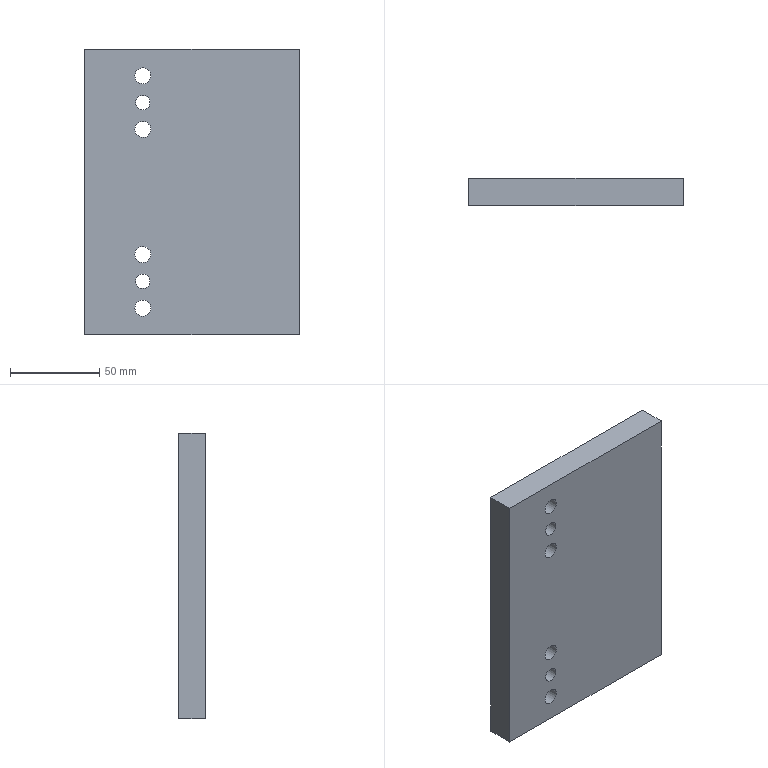Part | STEP file | Copy (1) of SN10_008_007-02_PLACA | 1 solid | 12 faces | box 120 x 15 x 160 mm | volume 282675 mm3 | cylinder 6 | plane 6 | commonest cylinder face diameters 9 x4 8 x2
STEP:
#1=CARTESIAN_POINT('',(0.,0.,0.));
#2=DIRECTION('',(0.,0.,1.));
#3=DIRECTION('',(1.,0.,0.));
#4=AXIS2_PLACEMENT_3D('',#1,#2,#3);
#5=CARTESIAN_POINT('',(279.639,240.,404.352));
#6=VERTEX_POINT('',#5);
#7=CARTESIAN_POINT('',(276.129,240.,406.27));
#8=DIRECTION('',(0.,-1.,0.));
#9=DIRECTION('',(1.,0.,0.));
#10=AXIS2_PLACEMENT_3D('',#7,#8,#9);
#11=CIRCLE('',#10,4.);
#12=CARTESIAN_POINT('',(276.129,240.1,406.27));
#13=DIRECTION('',(0.,1.,0.));
#14=DIRECTION('',(0.8776,0.,-0.4794));
#15=AXIS2_PLACEMENT_3D('',#12,#13,#14);
#16=CYLINDRICAL_SURFACE('',#15,4.);
#17=CARTESIAN_POINT('',(12.066,-0.1));
#18=DIRECTION('',(-1.,0.));
#19=VECTOR('',#18,1.);
#20=LINE('',#17,#19);
#21=(GEOMETRIC_REPRESENTATION_CONTEXT(2)PARAMETRIC_REPRESENTATION_CONTEXT()REPRESENTATION_CONTEXT('',''));
#22=DEFINITIONAL_REPRESENTATION('',(#20),#21);
#23=PCURVE('',#16,#22);
#24=CARTESIAN_POINT('',(363.629,240.,446.));
#25=DIRECTION('',(0.,-1.,0.));
#26=DIRECTION('',(0.,0.,-1.));
#27=AXIS2_PLACEMENT_3D('',#24,#25,#26);
#28=PLANE('',#27);
#29=CARTESIAN_POINT('',(39.73,-87.5));
#30=DIRECTION('',(0.,1.));
#31=AXIS2_PLACEMENT_2D('',#29,#30);
#32=CIRCLE('',#31,4.);
#33=(GEOMETRIC_REPRESENTATION_CONTEXT(2)PARAMETRIC_REPRESENTATION_CONTEXT()REPRESENTATION_CONTEXT('',''));
#34=DEFINITIONAL_REPRESENTATION('',(#32),#33);
#35=PCURVE('',#28,#34);
#36=SURFACE_CURVE('',#11,(#23,#35),.PCURVE_S1.);
#37=EDGE_CURVE('',#6,#6,#36,.T.);
#38=ORIENTED_EDGE('',*,*,#37,.F.);
#39=CARTESIAN_POINT('',(279.639,255.,404.352));
#40=VERTEX_POINT('',#39);
#41=CARTESIAN_POINT('',(279.639,240.,404.352));
#42=CARTESIAN_POINT('',(279.639,255.,404.352));
#43=B_SPLINE_CURVE_WITH_KNOTS('',1,(#41,#42),.UNSPECIFIED.,.F.,.F.,(2,2),(-0.1,14.9),.PIECEWISE_BEZIER_KNOTS.);
#44=CARTESIAN_POINT('',(6.283,0.));
#45=DIRECTION('',(0.,1.));
#46=VECTOR('',#45,1.);
#47=LINE('',#44,#46);
#48=(GEOMETRIC_REPRESENTATION_CONTEXT(2)PARAMETRIC_REPRESENTATION_CONTEXT()REPRESENTATION_CONTEXT('',''));
#49=DEFINITIONAL_REPRESENTATION('',(#47),#48);
#50=PCURVE('',#16,#49);
#51=CARTESIAN_POINT('',(0.,0.));
#52=DIRECTION('',(0.,1.));
#53=VECTOR('',#52,1.);
#54=LINE('',#51,#53);
#55=(GEOMETRIC_REPRESENTATION_CONTEXT(2)PARAMETRIC_REPRESENTATION_CONTEXT()REPRESENTATION_CONTEXT('',''));
#56=DEFINITIONAL_REPRESENTATION('',(#54),#55);
#57=PCURVE('',#16,#56);
#58=SEAM_CURVE('',#43,(#50,#57),.PCURVE_S1.);
#59=EDGE_CURVE('',#6,#40,#58,.T.);
#60=ORIENTED_EDGE('',*,*,#59,.T.);
#61=CARTESIAN_POINT('',(276.129,255.,406.27));
#62=DIRECTION('',(0.,1.,0.));
#63=DIRECTION('',(1.,0.,0.));
#64=AXIS2_PLACEMENT_3D('',#61,#62,#63);
#65=CIRCLE('',#64,4.);
#66=CARTESIAN_POINT('',(-0.5,14.9));
#67=DIRECTION('',(1.,0.));
#68=VECTOR('',#67,1.);
#69=LINE('',#66,#68);
#70=(GEOMETRIC_REPRESENTATION_CONTEXT(2)PARAMETRIC_REPRESENTATION_CONTEXT()REPRESENTATION_CONTEXT('',''));
#71=DEFINITIONAL_REPRESENTATION('',(#69),#70);
#72=PCURVE('',#16,#71);
#73=CARTESIAN_POINT('',(243.629,255.,446.));
#74=DIRECTION('',(0.,1.,0.));
#75=DIRECTION('',(0.,0.,1.));
#76=AXIS2_PLACEMENT_3D('',#73,#74,#75);
#77=PLANE('',#76);
#78=CARTESIAN_POINT('',(-39.73,32.5));
#79=DIRECTION('',(0.,1.));
#80=AXIS2_PLACEMENT_2D('',#78,#79);
#81=CIRCLE('',#80,4.);
#82=(GEOMETRIC_REPRESENTATION_CONTEXT(2)PARAMETRIC_REPRESENTATION_CONTEXT()REPRESENTATION_CONTEXT('',''));
#83=DEFINITIONAL_REPRESENTATION('',(#81),#82);
#84=PCURVE('',#77,#83);
#85=SURFACE_CURVE('',#65,(#72,#84),.PCURVE_S1.);
#86=EDGE_CURVE('',#40,#40,#85,.T.);
#87=ORIENTED_EDGE('',*,*,#86,.F.);
#88=ORIENTED_EDGE('',*,*,#59,.F.);
#89=EDGE_LOOP('',(#38,#60,#87,#88));
#90=FACE_BOUND('',#89,.F.);
#91=ADVANCED_FACE('',(#90),#16,.F.);
#92=CARTESIAN_POINT('',(243.629,240.,436.27));
#93=VERTEX_POINT('',#92);
#94=CARTESIAN_POINT('',(243.629,240.,276.27));
#95=VERTEX_POINT('',#94);
#96=CARTESIAN_POINT('',(243.629,240.,436.27));
#97=DIRECTION('',(0.,0.,-1.));
#98=VECTOR('',#97,1.);
#99=LINE('',#96,#98);
#100=CARTESIAN_POINT('',(9.73,-120.));
#101=DIRECTION('',(1.,0.));
#102=VECTOR('',#101,1.);
#103=LINE('',#100,#102);
#104=(GEOMETRIC_REPRESENTATION_CONTEXT(2)PARAMETRIC_REPRESENTATION_CONTEXT()REPRESENTATION_CONTEXT('',''));
#105=DEFINITIONAL_REPRESENTATION('',(#103),#104);
#106=PCURVE('',#28,#105);
#107=CARTESIAN_POINT('',(243.629,255.,446.));
#108=DIRECTION('',(1.,0.,0.));
#109=DIRECTION('',(0.,0.,-1.));
#110=AXIS2_PLACEMENT_3D('',#107,#108,#109);
#111=PLANE('',#110);
#112=CARTESIAN_POINT('',(9.73,-15.));
#113=DIRECTION('',(1.,0.));
#114=VECTOR('',#113,1.);
#115=LINE('',#112,#114);
#116=(GEOMETRIC_REPRESENTATION_CONTEXT(2)PARAMETRIC_REPRESENTATION_CONTEXT()REPRESENTATION_CONTEXT('',''));
#117=DEFINITIONAL_REPRESENTATION('',(#115),#116);
#118=PCURVE('',#111,#117);
#119=SURFACE_CURVE('',#99,(#106,#118),.PCURVE_S1.);
#120=EDGE_CURVE('',#93,#95,#119,.T.);
#121=ORIENTED_EDGE('',*,*,#120,.T.);
#122=CARTESIAN_POINT('',(363.629,240.,276.27));
#123=VERTEX_POINT('',#122);
#124=CARTESIAN_POINT('',(363.629,240.,276.27));
#125=DIRECTION('',(-1.,0.,0.));
#126=VECTOR('',#125,1.);
#127=LINE('',#124,#126);
#128=CARTESIAN_POINT('',(169.73,0.));
#129=DIRECTION('',(0.,-1.));
#130=VECTOR('',#129,1.);
#131=LINE('',#128,#130);
#132=(GEOMETRIC_REPRESENTATION_CONTEXT(2)PARAMETRIC_REPRESENTATION_CONTEXT()REPRESENTATION_CONTEXT('',''));
#133=DEFINITIONAL_REPRESENTATION('',(#131),#132);
#134=PCURVE('',#28,#133);
#135=CARTESIAN_POINT('',(243.629,270.,276.27));
#136=DIRECTION('',(0.,0.,-1.));
#137=DIRECTION('',(-1.,0.,0.));
#138=AXIS2_PLACEMENT_3D('',#135,#136,#137);
#139=PLANE('',#138);
#140=CARTESIAN_POINT('',(-120.,-30.));
#141=DIRECTION('',(1.,0.));
#142=VECTOR('',#141,1.);
#143=LINE('',#140,#142);
#144=(GEOMETRIC_REPRESENTATION_CONTEXT(2)PARAMETRIC_REPRESENTATION_CONTEXT()REPRESENTATION_CONTEXT('',''));
#145=DEFINITIONAL_REPRESENTATION('',(#143),#144);
#146=PCURVE('',#139,#145);
#147=SURFACE_CURVE('',#127,(#134,#146),.PCURVE_S1.);
#148=EDGE_CURVE('',#123,#95,#147,.T.);
#149=ORIENTED_EDGE('',*,*,#148,.F.);
#150=CARTESIAN_POINT('',(363.629,240.,436.27));
#151=VERTEX_POINT('',#150);
#152=CARTESIAN_POINT('',(363.629,240.,436.27));
#153=DIRECTION('',(0.,0.,-1.));
#154=VECTOR('',#153,1.);
#155=LINE('',#152,#154);
#156=CARTESIAN_POINT('',(9.73,0.));
#157=DIRECTION('',(1.,0.));
#158=VECTOR('',#157,1.);
#159=LINE('',#156,#158);
#160=(GEOMETRIC_REPRESENTATION_CONTEXT(2)PARAMETRIC_REPRESENTATION_CONTEXT()REPRESENTATION_CONTEXT('',''));
#161=DEFINITIONAL_REPRESENTATION('',(#159),#160);
#162=PCURVE('',#28,#161);
#163=CARTESIAN_POINT('',(363.629,240.,446.));
#164=DIRECTION('',(-1.,0.,0.));
#165=DIRECTION('',(0.,0.,1.));
#166=AXIS2_PLACEMENT_3D('',#163,#164,#165);
#167=PLANE('',#166);
#168=CARTESIAN_POINT('',(-9.73,0.));
#169=DIRECTION('',(-1.,0.));
#170=VECTOR('',#169,1.);
#171=LINE('',#168,#170);
#172=(GEOMETRIC_REPRESENTATION_CONTEXT(2)PARAMETRIC_REPRESENTATION_CONTEXT()REPRESENTATION_CONTEXT('',''));
#173=DEFINITIONAL_REPRESENTATION('',(#171),#172);
#174=PCURVE('',#167,#173);
#175=SURFACE_CURVE('',#155,(#162,#174),.PCURVE_S1.);
#176=EDGE_CURVE('',#151,#123,#175,.T.);
#177=ORIENTED_EDGE('',*,*,#176,.F.);
#178=CARTESIAN_POINT('',(363.629,240.,436.27));
#179=DIRECTION('',(-1.,0.,0.));
#180=VECTOR('',#179,1.);
#181=LINE('',#178,#180);
#182=CARTESIAN_POINT('',(9.73,0.));
#183=DIRECTION('',(0.,-1.));
#184=VECTOR('',#183,1.);
#185=LINE('',#182,#184);
#186=(GEOMETRIC_REPRESENTATION_CONTEXT(2)PARAMETRIC_REPRESENTATION_CONTEXT()REPRESENTATION_CONTEXT('',''));
#187=DEFINITIONAL_REPRESENTATION('',(#185),#186);
#188=PCURVE('',#28,#187);
#189=CARTESIAN_POINT('',(243.629,255.,436.27));
#190=DIRECTION('',(0.,0.,1.));
#191=DIRECTION('',(1.,0.,0.));
#192=AXIS2_PLACEMENT_3D('',#189,#190,#191);
#193=PLANE('',#192);
#194=CARTESIAN_POINT('',(120.,-15.));
#195=DIRECTION('',(-1.,0.));
#196=VECTOR('',#195,1.);
#197=LINE('',#194,#196);
#198=(GEOMETRIC_REPRESENTATION_CONTEXT(2)PARAMETRIC_REPRESENTATION_CONTEXT()REPRESENTATION_CONTEXT('',''));
#199=DEFINITIONAL_REPRESENTATION('',(#197),#198);
#200=PCURVE('',#193,#199);
#201=SURFACE_CURVE('',#181,(#188,#200),.PCURVE_S1.);
#202=EDGE_CURVE('',#151,#93,#201,.T.);
#203=ORIENTED_EDGE('',*,*,#202,.T.);
#204=EDGE_LOOP('',(#121,#149,#177,#203));
#205=FACE_BOUND('',#204,.T.);
#206=ORIENTED_EDGE('',*,*,#37,.F.);
#207=EDGE_LOOP('',(#206));
#208=FACE_BOUND('',#207,.T.);
#209=CARTESIAN_POINT('',(279.639,240.,304.352));
#210=VERTEX_POINT('',#209);
#211=CARTESIAN_POINT('',(276.129,240.,306.27));
#212=DIRECTION('',(0.,-1.,0.));
#213=DIRECTION('',(1.,0.,0.));
#214=AXIS2_PLACEMENT_3D('',#211,#212,#213);
#215=CIRCLE('',#214,4.);
#216=CARTESIAN_POINT('',(139.73,-87.5));
#217=DIRECTION('',(0.,1.));
#218=AXIS2_PLACEMENT_2D('',#216,#217);
#219=CIRCLE('',#218,4.);
#220=(GEOMETRIC_REPRESENTATION_CONTEXT(2)PARAMETRIC_REPRESENTATION_CONTEXT()REPRESENTATION_CONTEXT('',''));
#221=DEFINITIONAL_REPRESENTATION('',(#219),#220);
#222=PCURVE('',#28,#221);
#223=CARTESIAN_POINT('',(276.129,240.1,306.27));
#224=DIRECTION('',(0.,1.,0.));
#225=DIRECTION('',(0.8776,0.,-0.4794));
#226=AXIS2_PLACEMENT_3D('',#223,#224,#225);
#227=CYLINDRICAL_SURFACE('',#226,4.);
#228=CARTESIAN_POINT('',(12.066,-0.1));
#229=DIRECTION('',(-1.,0.));
#230=VECTOR('',#229,1.);
#231=LINE('',#228,#230);
#232=(GEOMETRIC_REPRESENTATION_CONTEXT(2)PARAMETRIC_REPRESENTATION_CONTEXT()REPRESENTATION_CONTEXT('',''));
#233=DEFINITIONAL_REPRESENTATION('',(#231),#232);
#234=PCURVE('',#227,#233);
#235=SURFACE_CURVE('',#215,(#222,#234),.PCURVE_S1.);
#236=EDGE_CURVE('',#210,#210,#235,.T.);
#237=ORIENTED_EDGE('',*,*,#236,.F.);
#238=EDGE_LOOP('',(#237));
#239=FACE_BOUND('',#238,.T.);
#240=CARTESIAN_POINT('',(280.078,240.,319.113));
#241=VERTEX_POINT('',#240);
#242=CARTESIAN_POINT('',(276.129,240.,321.27));
#243=DIRECTION('',(0.,-1.,0.));
#244=DIRECTION('',(1.,0.,0.));
#245=AXIS2_PLACEMENT_3D('',#242,#243,#244);
#246=CIRCLE('',#245,4.5);
#247=CARTESIAN_POINT('',(124.73,-87.5));
#248=DIRECTION('',(0.,1.));
#249=AXIS2_PLACEMENT_2D('',#247,#248);
#250=CIRCLE('',#249,4.5);
#251=(GEOMETRIC_REPRESENTATION_CONTEXT(2)PARAMETRIC_REPRESENTATION_CONTEXT()REPRESENTATION_CONTEXT('',''));
#252=DEFINITIONAL_REPRESENTATION('',(#250),#251);
#253=PCURVE('',#28,#252);
#254=CARTESIAN_POINT('',(276.129,240.1,321.27));
#255=DIRECTION('',(0.,1.,0.));
#256=DIRECTION('',(0.8776,0.,-0.4794));
#257=AXIS2_PLACEMENT_3D('',#254,#255,#256);
#258=CYLINDRICAL_SURFACE('',#257,4.5);
#259=CARTESIAN_POINT('',(12.066,-0.1));
#260=DIRECTION('',(-1.,0.));
#261=VECTOR('',#260,1.);
#262=LINE('',#259,#261);
#263=(GEOMETRIC_REPRESENTATION_CONTEXT(2)PARAMETRIC_REPRESENTATION_CONTEXT()REPRESENTATION_CONTEXT('',''));
#264=DEFINITIONAL_REPRESENTATION('',(#262),#263);
#265=PCURVE('',#258,#264);
#266=SURFACE_CURVE('',#246,(#253,#265),.PCURVE_S1.);
#267=EDGE_CURVE('',#241,#241,#266,.T.);
#268=ORIENTED_EDGE('',*,*,#267,.F.);
#269=EDGE_LOOP('',(#268));
#270=FACE_BOUND('',#269,.T.);
#271=CARTESIAN_POINT('',(280.078,240.,289.113));
#272=VERTEX_POINT('',#271);
#273=CARTESIAN_POINT('',(276.129,240.,291.27));
#274=DIRECTION('',(0.,-1.,0.));
#275=DIRECTION('',(1.,0.,0.));
#276=AXIS2_PLACEMENT_3D('',#273,#274,#275);
#277=CIRCLE('',#276,4.5);
#278=CARTESIAN_POINT('',(154.73,-87.5));
#279=DIRECTION('',(0.,1.));
#280=AXIS2_PLACEMENT_2D('',#278,#279);
#281=CIRCLE('',#280,4.5);
#282=(GEOMETRIC_REPRESENTATION_CONTEXT(2)PARAMETRIC_REPRESENTATION_CONTEXT()REPRESENTATION_CONTEXT('',''));
#283=DEFINITIONAL_REPRESENTATION('',(#281),#282);
#284=PCURVE('',#28,#283);
#285=CARTESIAN_POINT('',(276.129,240.1,291.27));
#286=DIRECTION('',(0.,1.,0.));
#287=DIRECTION('',(0.8776,0.,-0.4794));
#288=AXIS2_PLACEMENT_3D('',#285,#286,#287);
#289=CYLINDRICAL_SURFACE('',#288,4.5);
#290=CARTESIAN_POINT('',(12.066,-0.1));
#291=DIRECTION('',(-1.,0.));
#292=VECTOR('',#291,1.);
#293=LINE('',#290,#292);
#294=(GEOMETRIC_REPRESENTATION_CONTEXT(2)PARAMETRIC_REPRESENTATION_CONTEXT()REPRESENTATION_CONTEXT('',''));
#295=DEFINITIONAL_REPRESENTATION('',(#293),#294);
#296=PCURVE('',#289,#295);
#297=SURFACE_CURVE('',#277,(#284,#296),.PCURVE_S1.);
#298=EDGE_CURVE('',#272,#272,#297,.T.);
#299=ORIENTED_EDGE('',*,*,#298,.F.);
#300=EDGE_LOOP('',(#299));
#301=FACE_BOUND('',#300,.T.);
#302=CARTESIAN_POINT('',(280.078,240.,389.113));
#303=VERTEX_POINT('',#302);
#304=CARTESIAN_POINT('',(276.129,240.,391.27));
#305=DIRECTION('',(0.,-1.,0.));
#306=DIRECTION('',(1.,0.,0.));
#307=AXIS2_PLACEMENT_3D('',#304,#305,#306);
#308=CIRCLE('',#307,4.5);
#309=CARTESIAN_POINT('',(54.73,-87.5));
#310=DIRECTION('',(0.,1.));
#311=AXIS2_PLACEMENT_2D('',#309,#310);
#312=CIRCLE('',#311,4.5);
#313=(GEOMETRIC_REPRESENTATION_CONTEXT(2)PARAMETRIC_REPRESENTATION_CONTEXT()REPRESENTATION_CONTEXT('',''));
#314=DEFINITIONAL_REPRESENTATION('',(#312),#313);
#315=PCURVE('',#28,#314);
#316=CARTESIAN_POINT('',(276.129,240.1,391.27));
#317=DIRECTION('',(0.,1.,0.));
#318=DIRECTION('',(0.8776,0.,-0.4794));
#319=AXIS2_PLACEMENT_3D('',#316,#317,#318);
#320=CYLINDRICAL_SURFACE('',#319,4.5);
#321=CARTESIAN_POINT('',(12.066,-0.1));
#322=DIRECTION('',(-1.,0.));
#323=VECTOR('',#322,1.);
#324=LINE('',#321,#323);
#325=(GEOMETRIC_REPRESENTATION_CONTEXT(2)PARAMETRIC_REPRESENTATION_CONTEXT()REPRESENTATION_CONTEXT('',''));
#326=DEFINITIONAL_REPRESENTATION('',(#324),#325);
#327=PCURVE('',#320,#326);
#328=SURFACE_CURVE('',#308,(#315,#327),.PCURVE_S1.);
#329=EDGE_CURVE('',#303,#303,#328,.T.);
#330=ORIENTED_EDGE('',*,*,#329,.F.);
#331=EDGE_LOOP('',(#330));
#332=FACE_BOUND('',#331,.T.);
#333=CARTESIAN_POINT('',(280.078,240.,419.113));
#334=VERTEX_POINT('',#333);
#335=CARTESIAN_POINT('',(276.129,240.,421.27));
#336=DIRECTION('',(0.,-1.,0.));
#337=DIRECTION('',(1.,0.,0.));
#338=AXIS2_PLACEMENT_3D('',#335,#336,#337);
#339=CIRCLE('',#338,4.5);
#340=CARTESIAN_POINT('',(24.73,-87.5));
#341=DIRECTION('',(0.,1.));
#342=AXIS2_PLACEMENT_2D('',#340,#341);
#343=CIRCLE('',#342,4.5);
#344=(GEOMETRIC_REPRESENTATION_CONTEXT(2)PARAMETRIC_REPRESENTATION_CONTEXT()REPRESENTATION_CONTEXT('',''));
#345=DEFINITIONAL_REPRESENTATION('',(#343),#344);
#346=PCURVE('',#28,#345);
#347=CARTESIAN_POINT('',(276.129,240.1,421.27));
#348=DIRECTION('',(0.,1.,0.));
#349=DIRECTION('',(0.8776,0.,-0.4794));
#350=AXIS2_PLACEMENT_3D('',#347,#348,#349);
#351=CYLINDRICAL_SURFACE('',#350,4.5);
#352=CARTESIAN_POINT('',(12.066,-0.1));
#353=DIRECTION('',(-1.,0.));
#354=VECTOR('',#353,1.);
#355=LINE('',#352,#354);
#356=(GEOMETRIC_REPRESENTATION_CONTEXT(2)PARAMETRIC_REPRESENTATION_CONTEXT()REPRESENTATION_CONTEXT('',''));
#357=DEFINITIONAL_REPRESENTATION('',(#355),#356);
#358=PCURVE('',#351,#357);
#359=SURFACE_CURVE('',#339,(#346,#358),.PCURVE_S1.);
#360=EDGE_CURVE('',#334,#334,#359,.T.);
#361=ORIENTED_EDGE('',*,*,#360,.F.);
#362=EDGE_LOOP('',(#361));
#363=FACE_BOUND('',#362,.T.);
#364=ADVANCED_FACE('',(#205,#208,#239,#270,#301,#332,#363),#28,.T.);
#365=CARTESIAN_POINT('',(363.629,255.,436.27));
#366=VERTEX_POINT('',#365);
#367=CARTESIAN_POINT('',(363.629,255.,276.27));
#368=VERTEX_POINT('',#367);
#369=CARTESIAN_POINT('',(363.629,255.,436.27));
#370=DIRECTION('',(0.,0.,-1.));
#371=VECTOR('',#370,1.);
#372=LINE('',#369,#371);
#373=CARTESIAN_POINT('',(-9.73,120.));
#374=DIRECTION('',(-1.,0.));
#375=VECTOR('',#374,1.);
#376=LINE('',#373,#375);
#377=(GEOMETRIC_REPRESENTATION_CONTEXT(2)PARAMETRIC_REPRESENTATION_CONTEXT()REPRESENTATION_CONTEXT('',''));
#378=DEFINITIONAL_REPRESENTATION('',(#376),#377);
#379=PCURVE('',#77,#378);
#380=CARTESIAN_POINT('',(-9.73,15.));
#381=DIRECTION('',(-1.,0.));
#382=VECTOR('',#381,1.);
#383=LINE('',#380,#382);
#384=(GEOMETRIC_REPRESENTATION_CONTEXT(2)PARAMETRIC_REPRESENTATION_CONTEXT()REPRESENTATION_CONTEXT('',''));
#385=DEFINITIONAL_REPRESENTATION('',(#383),#384);
#386=PCURVE('',#167,#385);
#387=SURFACE_CURVE('',#372,(#379,#386),.PCURVE_S1.);
#388=EDGE_CURVE('',#366,#368,#387,.T.);
#389=ORIENTED_EDGE('',*,*,#388,.T.);
#390=CARTESIAN_POINT('',(243.629,255.,276.27));
#391=VERTEX_POINT('',#390);
#392=CARTESIAN_POINT('',(243.629,255.,276.27));
#393=DIRECTION('',(1.,0.,0.));
#394=VECTOR('',#393,1.);
#395=LINE('',#392,#394);
#396=CARTESIAN_POINT('',(-169.73,0.));
#397=DIRECTION('',(0.,1.));
#398=VECTOR('',#397,1.);
#399=LINE('',#396,#398);
#400=(GEOMETRIC_REPRESENTATION_CONTEXT(2)PARAMETRIC_REPRESENTATION_CONTEXT()REPRESENTATION_CONTEXT('',''));
#401=DEFINITIONAL_REPRESENTATION('',(#399),#400);
#402=PCURVE('',#77,#401);
#403=CARTESIAN_POINT('',(0.,-15.));
#404=DIRECTION('',(-1.,0.));
#405=VECTOR('',#404,1.);
#406=LINE('',#403,#405);
#407=(GEOMETRIC_REPRESENTATION_CONTEXT(2)PARAMETRIC_REPRESENTATION_CONTEXT()REPRESENTATION_CONTEXT('',''));
#408=DEFINITIONAL_REPRESENTATION('',(#406),#407);
#409=PCURVE('',#139,#408);
#410=SURFACE_CURVE('',#395,(#402,#409),.PCURVE_S1.);
#411=EDGE_CURVE('',#391,#368,#410,.T.);
#412=ORIENTED_EDGE('',*,*,#411,.F.);
#413=CARTESIAN_POINT('',(243.629,255.,436.27));
#414=VERTEX_POINT('',#413);
#415=CARTESIAN_POINT('',(243.629,255.,436.27));
#416=DIRECTION('',(0.,0.,-1.));
#417=VECTOR('',#416,1.);
#418=LINE('',#415,#417);
#419=CARTESIAN_POINT('',(-9.73,0.));
#420=DIRECTION('',(-1.,0.));
#421=VECTOR('',#420,1.);
#422=LINE('',#419,#421);
#423=(GEOMETRIC_REPRESENTATION_CONTEXT(2)PARAMETRIC_REPRESENTATION_CONTEXT()REPRESENTATION_CONTEXT('',''));
#424=DEFINITIONAL_REPRESENTATION('',(#422),#423);
#425=PCURVE('',#77,#424);
#426=CARTESIAN_POINT('',(9.73,0.));
#427=DIRECTION('',(1.,0.));
#428=VECTOR('',#427,1.);
#429=LINE('',#426,#428);
#430=(GEOMETRIC_REPRESENTATION_CONTEXT(2)PARAMETRIC_REPRESENTATION_CONTEXT()REPRESENTATION_CONTEXT('',''));
#431=DEFINITIONAL_REPRESENTATION('',(#429),#430);
#432=PCURVE('',#111,#431);
#433=SURFACE_CURVE('',#418,(#425,#432),.PCURVE_S1.);
#434=EDGE_CURVE('',#414,#391,#433,.T.);
#435=ORIENTED_EDGE('',*,*,#434,.F.);
#436=CARTESIAN_POINT('',(243.629,255.,436.27));
#437=DIRECTION('',(1.,0.,0.));
#438=VECTOR('',#437,1.);
#439=LINE('',#436,#438);
#440=CARTESIAN_POINT('',(-9.73,0.));
#441=DIRECTION('',(0.,1.));
#442=VECTOR('',#441,1.);
#443=LINE('',#440,#442);
#444=(GEOMETRIC_REPRESENTATION_CONTEXT(2)PARAMETRIC_REPRESENTATION_CONTEXT()REPRESENTATION_CONTEXT('',''));
#445=DEFINITIONAL_REPRESENTATION('',(#443),#444);
#446=PCURVE('',#77,#445);
#447=CARTESIAN_POINT('',(0.,0.));
#448=DIRECTION('',(1.,0.));
#449=VECTOR('',#448,1.);
#450=LINE('',#447,#449);
#451=(GEOMETRIC_REPRESENTATION_CONTEXT(2)PARAMETRIC_REPRESENTATION_CONTEXT()REPRESENTATION_CONTEXT('',''));
#452=DEFINITIONAL_REPRESENTATION('',(#450),#451);
#453=PCURVE('',#193,#452);
#454=SURFACE_CURVE('',#439,(#446,#453),.PCURVE_S1.);
#455=EDGE_CURVE('',#414,#366,#454,.T.);
#456=ORIENTED_EDGE('',*,*,#455,.T.);
#457=EDGE_LOOP('',(#389,#412,#435,#456));
#458=FACE_BOUND('',#457,.T.);
#459=ORIENTED_EDGE('',*,*,#86,.F.);
#460=EDGE_LOOP('',(#459));
#461=FACE_BOUND('',#460,.T.);
#462=CARTESIAN_POINT('',(279.639,255.,304.352));
#463=VERTEX_POINT('',#462);
#464=CARTESIAN_POINT('',(276.129,255.,306.27));
#465=DIRECTION('',(0.,1.,0.));
#466=DIRECTION('',(1.,0.,0.));
#467=AXIS2_PLACEMENT_3D('',#464,#465,#466);
#468=CIRCLE('',#467,4.);
#469=CARTESIAN_POINT('',(-139.73,32.5));
#470=DIRECTION('',(0.,1.));
#471=AXIS2_PLACEMENT_2D('',#469,#470);
#472=CIRCLE('',#471,4.);
#473=(GEOMETRIC_REPRESENTATION_CONTEXT(2)PARAMETRIC_REPRESENTATION_CONTEXT()REPRESENTATION_CONTEXT('',''));
#474=DEFINITIONAL_REPRESENTATION('',(#472),#473);
#475=PCURVE('',#77,#474);
#476=CARTESIAN_POINT('',(-0.5,14.9));
#477=DIRECTION('',(1.,0.));
#478=VECTOR('',#477,1.);
#479=LINE('',#476,#478);
#480=(GEOMETRIC_REPRESENTATION_CONTEXT(2)PARAMETRIC_REPRESENTATION_CONTEXT()REPRESENTATION_CONTEXT('',''));
#481=DEFINITIONAL_REPRESENTATION('',(#479),#480);
#482=PCURVE('',#227,#481);
#483=SURFACE_CURVE('',#468,(#475,#482),.PCURVE_S1.);
#484=EDGE_CURVE('',#463,#463,#483,.T.);
#485=ORIENTED_EDGE('',*,*,#484,.F.);
#486=EDGE_LOOP('',(#485));
#487=FACE_BOUND('',#486,.T.);
#488=CARTESIAN_POINT('',(280.078,255.,319.113));
#489=VERTEX_POINT('',#488);
#490=CARTESIAN_POINT('',(276.129,255.,321.27));
#491=DIRECTION('',(0.,1.,0.));
#492=DIRECTION('',(1.,0.,0.));
#493=AXIS2_PLACEMENT_3D('',#490,#491,#492);
#494=CIRCLE('',#493,4.5);
#495=CARTESIAN_POINT('',(-124.73,32.5));
#496=DIRECTION('',(0.,1.));
#497=AXIS2_PLACEMENT_2D('',#495,#496);
#498=CIRCLE('',#497,4.5);
#499=(GEOMETRIC_REPRESENTATION_CONTEXT(2)PARAMETRIC_REPRESENTATION_CONTEXT()REPRESENTATION_CONTEXT('',''));
#500=DEFINITIONAL_REPRESENTATION('',(#498),#499);
#501=PCURVE('',#77,#500);
#502=CARTESIAN_POINT('',(-0.5,14.9));
#503=DIRECTION('',(1.,0.));
#504=VECTOR('',#503,1.);
#505=LINE('',#502,#504);
#506=(GEOMETRIC_REPRESENTATION_CONTEXT(2)PARAMETRIC_REPRESENTATION_CONTEXT()REPRESENTATION_CONTEXT('',''));
#507=DEFINITIONAL_REPRESENTATION('',(#505),#506);
#508=PCURVE('',#258,#507);
#509=SURFACE_CURVE('',#494,(#501,#508),.PCURVE_S1.);
#510=EDGE_CURVE('',#489,#489,#509,.T.);
#511=ORIENTED_EDGE('',*,*,#510,.F.);
#512=EDGE_LOOP('',(#511));
#513=FACE_BOUND('',#512,.T.);
#514=CARTESIAN_POINT('',(280.078,255.,289.113));
#515=VERTEX_POINT('',#514);
#516=CARTESIAN_POINT('',(276.129,255.,291.27));
#517=DIRECTION('',(0.,1.,0.));
#518=DIRECTION('',(1.,0.,0.));
#519=AXIS2_PLACEMENT_3D('',#516,#517,#518);
#520=CIRCLE('',#519,4.5);
#521=CARTESIAN_POINT('',(-154.73,32.5));
#522=DIRECTION('',(0.,1.));
#523=AXIS2_PLACEMENT_2D('',#521,#522);
#524=CIRCLE('',#523,4.5);
#525=(GEOMETRIC_REPRESENTATION_CONTEXT(2)PARAMETRIC_REPRESENTATION_CONTEXT()REPRESENTATION_CONTEXT('',''));
#526=DEFINITIONAL_REPRESENTATION('',(#524),#525);
#527=PCURVE('',#77,#526);
#528=CARTESIAN_POINT('',(-0.5,14.9));
#529=DIRECTION('',(1.,0.));
#530=VECTOR('',#529,1.);
#531=LINE('',#528,#530);
#532=(GEOMETRIC_REPRESENTATION_CONTEXT(2)PARAMETRIC_REPRESENTATION_CONTEXT()REPRESENTATION_CONTEXT('',''));
#533=DEFINITIONAL_REPRESENTATION('',(#531),#532);
#534=PCURVE('',#289,#533);
#535=SURFACE_CURVE('',#520,(#527,#534),.PCURVE_S1.);
#536=EDGE_CURVE('',#515,#515,#535,.T.);
#537=ORIENTED_EDGE('',*,*,#536,.F.);
#538=EDGE_LOOP('',(#537));
#539=FACE_BOUND('',#538,.T.);
#540=CARTESIAN_POINT('',(280.078,255.,389.113));
#541=VERTEX_POINT('',#540);
#542=CARTESIAN_POINT('',(276.129,255.,391.27));
#543=DIRECTION('',(0.,1.,0.));
#544=DIRECTION('',(1.,0.,0.));
#545=AXIS2_PLACEMENT_3D('',#542,#543,#544);
#546=CIRCLE('',#545,4.5);
#547=CARTESIAN_POINT('',(-54.73,32.5));
#548=DIRECTION('',(0.,1.));
#549=AXIS2_PLACEMENT_2D('',#547,#548);
#550=CIRCLE('',#549,4.5);
#551=(GEOMETRIC_REPRESENTATION_CONTEXT(2)PARAMETRIC_REPRESENTATION_CONTEXT()REPRESENTATION_CONTEXT('',''));
#552=DEFINITIONAL_REPRESENTATION('',(#550),#551);
#553=PCURVE('',#77,#552);
#554=CARTESIAN_POINT('',(-0.5,14.9));
#555=DIRECTION('',(1.,0.));
#556=VECTOR('',#555,1.);
#557=LINE('',#554,#556);
#558=(GEOMETRIC_REPRESENTATION_CONTEXT(2)PARAMETRIC_REPRESENTATION_CONTEXT()REPRESENTATION_CONTEXT('',''));
#559=DEFINITIONAL_REPRESENTATION('',(#557),#558);
#560=PCURVE('',#320,#559);
#561=SURFACE_CURVE('',#546,(#553,#560),.PCURVE_S1.);
#562=EDGE_CURVE('',#541,#541,#561,.T.);
#563=ORIENTED_EDGE('',*,*,#562,.F.);
#564=EDGE_LOOP('',(#563));
#565=FACE_BOUND('',#564,.T.);
#566=CARTESIAN_POINT('',(280.078,255.,419.113));
#567=VERTEX_POINT('',#566);
#568=CARTESIAN_POINT('',(276.129,255.,421.27));
#569=DIRECTION('',(0.,1.,0.));
#570=DIRECTION('',(1.,0.,0.));
#571=AXIS2_PLACEMENT_3D('',#568,#569,#570);
#572=CIRCLE('',#571,4.5);
#573=CARTESIAN_POINT('',(-24.73,32.5));
#574=DIRECTION('',(0.,1.));
#575=AXIS2_PLACEMENT_2D('',#573,#574);
#576=CIRCLE('',#575,4.5);
#577=(GEOMETRIC_REPRESENTATION_CONTEXT(2)PARAMETRIC_REPRESENTATION_CONTEXT()REPRESENTATION_CONTEXT('',''));
#578=DEFINITIONAL_REPRESENTATION('',(#576),#577);
#579=PCURVE('',#77,#578);
#580=CARTESIAN_POINT('',(-0.5,14.9));
#581=DIRECTION('',(1.,0.));
#582=VECTOR('',#581,1.);
#583=LINE('',#580,#582);
#584=(GEOMETRIC_REPRESENTATION_CONTEXT(2)PARAMETRIC_REPRESENTATION_CONTEXT()REPRESENTATION_CONTEXT('',''));
#585=DEFINITIONAL_REPRESENTATION('',(#583),#584);
#586=PCURVE('',#351,#585);
#587=SURFACE_CURVE('',#572,(#579,#586),.PCURVE_S1.);
#588=EDGE_CURVE('',#567,#567,#587,.T.);
#589=ORIENTED_EDGE('',*,*,#588,.F.);
#590=EDGE_LOOP('',(#589));
#591=FACE_BOUND('',#590,.T.);
#592=ADVANCED_FACE('',(#458,#461,#487,#513,#539,#565,#591),#77,.T.);
#593=CARTESIAN_POINT('',(243.629,255.,436.27));
#594=DIRECTION('',(0.,-1.,0.));
#595=VECTOR('',#594,1.);
#596=LINE('',#593,#595);
#597=CARTESIAN_POINT('',(9.73,0.));
#598=DIRECTION('',(0.,-1.));
#599=VECTOR('',#598,1.);
#600=LINE('',#597,#599);
#601=(GEOMETRIC_REPRESENTATION_CONTEXT(2)PARAMETRIC_REPRESENTATION_CONTEXT()REPRESENTATION_CONTEXT('',''));
#602=DEFINITIONAL_REPRESENTATION('',(#600),#601);
#603=PCURVE('',#111,#602);
#604=CARTESIAN_POINT('',(0.,0.));
#605=DIRECTION('',(0.,-1.));
#606=VECTOR('',#605,1.);
#607=LINE('',#604,#606);
#608=(GEOMETRIC_REPRESENTATION_CONTEXT(2)PARAMETRIC_REPRESENTATION_CONTEXT()REPRESENTATION_CONTEXT('',''));
#609=DEFINITIONAL_REPRESENTATION('',(#607),#608);
#610=PCURVE('',#193,#609);
#611=SURFACE_CURVE('',#596,(#603,#610),.PCURVE_S1.);
#612=EDGE_CURVE('',#414,#93,#611,.T.);
#613=ORIENTED_EDGE('',*,*,#612,.F.);
#614=ORIENTED_EDGE('',*,*,#434,.T.);
#615=CARTESIAN_POINT('',(243.629,255.,276.27));
#616=DIRECTION('',(0.,-1.,0.));
#617=VECTOR('',#616,1.);
#618=LINE('',#615,#617);
#619=CARTESIAN_POINT('',(169.73,0.));
#620=DIRECTION('',(0.,-1.));
#621=VECTOR('',#620,1.);
#622=LINE('',#619,#621);
#623=(GEOMETRIC_REPRESENTATION_CONTEXT(2)PARAMETRIC_REPRESENTATION_CONTEXT()REPRESENTATION_CONTEXT('',''));
#624=DEFINITIONAL_REPRESENTATION('',(#622),#623);
#625=PCURVE('',#111,#624);
#626=CARTESIAN_POINT('',(0.,-15.));
#627=DIRECTION('',(0.,-1.));
#628=VECTOR('',#627,1.);
#629=LINE('',#626,#628);
#630=(GEOMETRIC_REPRESENTATION_CONTEXT(2)PARAMETRIC_REPRESENTATION_CONTEXT()REPRESENTATION_CONTEXT('',''));
#631=DEFINITIONAL_REPRESENTATION('',(#629),#630);
#632=PCURVE('',#139,#631);
#633=SURFACE_CURVE('',#618,(#625,#632),.PCURVE_S1.);
#634=EDGE_CURVE('',#391,#95,#633,.T.);
#635=ORIENTED_EDGE('',*,*,#634,.T.);
#636=ORIENTED_EDGE('',*,*,#120,.F.);
#637=EDGE_LOOP('',(#613,#614,#635,#636));
#638=FACE_BOUND('',#637,.T.);
#639=ADVANCED_FACE('',(#638),#111,.F.);
#640=ORIENTED_EDGE('',*,*,#455,.F.);
#641=ORIENTED_EDGE('',*,*,#612,.T.);
#642=ORIENTED_EDGE('',*,*,#202,.F.);
#643=CARTESIAN_POINT('',(363.629,255.,436.27));
#644=DIRECTION('',(0.,-1.,0.));
#645=VECTOR('',#644,1.);
#646=LINE('',#643,#645);
#647=CARTESIAN_POINT('',(120.,0.));
#648=DIRECTION('',(0.,-1.));
#649=VECTOR('',#648,1.);
#650=LINE('',#647,#649);
#651=(GEOMETRIC_REPRESENTATION_CONTEXT(2)PARAMETRIC_REPRESENTATION_CONTEXT()REPRESENTATION_CONTEXT('',''));
#652=DEFINITIONAL_REPRESENTATION('',(#650),#651);
#653=PCURVE('',#193,#652);
#654=CARTESIAN_POINT('',(-9.73,15.));
#655=DIRECTION('',(0.,-1.));
#656=VECTOR('',#655,1.);
#657=LINE('',#654,#656);
#658=(GEOMETRIC_REPRESENTATION_CONTEXT(2)PARAMETRIC_REPRESENTATION_CONTEXT()REPRESENTATION_CONTEXT('',''));
#659=DEFINITIONAL_REPRESENTATION('',(#657),#658);
#660=PCURVE('',#167,#659);
#661=SURFACE_CURVE('',#646,(#653,#660),.PCURVE_S1.);
#662=EDGE_CURVE('',#366,#151,#661,.T.);
#663=ORIENTED_EDGE('',*,*,#662,.F.);
#664=EDGE_LOOP('',(#640,#641,#642,#663));
#665=FACE_BOUND('',#664,.T.);
#666=ADVANCED_FACE('',(#665),#193,.T.);
#667=ORIENTED_EDGE('',*,*,#360,.F.);
#668=CARTESIAN_POINT('',(280.078,240.,419.113));
#669=CARTESIAN_POINT('',(280.078,255.,419.113));
#670=B_SPLINE_CURVE_WITH_KNOTS('',1,(#668,#669),.UNSPECIFIED.,.F.,.F.,(2,2),(-0.1,14.9),.PIECEWISE_BEZIER_KNOTS.);
#671=CARTESIAN_POINT('',(6.283,0.));
#672=DIRECTION('',(0.,1.));
#673=VECTOR('',#672,1.);
#674=LINE('',#671,#673);
#675=(GEOMETRIC_REPRESENTATION_CONTEXT(2)PARAMETRIC_REPRESENTATION_CONTEXT()REPRESENTATION_CONTEXT('',''));
#676=DEFINITIONAL_REPRESENTATION('',(#674),#675);
#677=PCURVE('',#351,#676);
#678=CARTESIAN_POINT('',(0.,0.));
#679=DIRECTION('',(0.,1.));
#680=VECTOR('',#679,1.);
#681=LINE('',#678,#680);
#682=(GEOMETRIC_REPRESENTATION_CONTEXT(2)PARAMETRIC_REPRESENTATION_CONTEXT()REPRESENTATION_CONTEXT('',''));
#683=DEFINITIONAL_REPRESENTATION('',(#681),#682);
#684=PCURVE('',#351,#683);
#685=SEAM_CURVE('',#670,(#677,#684),.PCURVE_S1.);
#686=EDGE_CURVE('',#334,#567,#685,.T.);
#687=ORIENTED_EDGE('',*,*,#686,.T.);
#688=ORIENTED_EDGE('',*,*,#588,.F.);
#689=ORIENTED_EDGE('',*,*,#686,.F.);
#690=EDGE_LOOP('',(#667,#687,#688,#689));
#691=FACE_BOUND('',#690,.F.);
#692=ADVANCED_FACE('',(#691),#351,.F.);
#693=ORIENTED_EDGE('',*,*,#329,.F.);
#694=CARTESIAN_POINT('',(280.078,240.,389.113));
#695=CARTESIAN_POINT('',(280.078,255.,389.113));
#696=B_SPLINE_CURVE_WITH_KNOTS('',1,(#694,#695),.UNSPECIFIED.,.F.,.F.,(2,2),(-0.1,14.9),.PIECEWISE_BEZIER_KNOTS.);
#697=CARTESIAN_POINT('',(6.283,0.));
#698=DIRECTION('',(0.,1.));
#699=VECTOR('',#698,1.);
#700=LINE('',#697,#699);
#701=(GEOMETRIC_REPRESENTATION_CONTEXT(2)PARAMETRIC_REPRESENTATION_CONTEXT()REPRESENTATION_CONTEXT('',''));
#702=DEFINITIONAL_REPRESENTATION('',(#700),#701);
#703=PCURVE('',#320,#702);
#704=CARTESIAN_POINT('',(0.,0.));
#705=DIRECTION('',(0.,1.));
#706=VECTOR('',#705,1.);
#707=LINE('',#704,#706);
#708=(GEOMETRIC_REPRESENTATION_CONTEXT(2)PARAMETRIC_REPRESENTATION_CONTEXT()REPRESENTATION_CONTEXT('',''));
#709=DEFINITIONAL_REPRESENTATION('',(#707),#708);
#710=PCURVE('',#320,#709);
#711=SEAM_CURVE('',#696,(#703,#710),.PCURVE_S1.);
#712=EDGE_CURVE('',#303,#541,#711,.T.);
#713=ORIENTED_EDGE('',*,*,#712,.T.);
#714=ORIENTED_EDGE('',*,*,#562,.F.);
#715=ORIENTED_EDGE('',*,*,#712,.F.);
#716=EDGE_LOOP('',(#693,#713,#714,#715));
#717=FACE_BOUND('',#716,.F.);
#718=ADVANCED_FACE('',(#717),#320,.F.);
#719=ORIENTED_EDGE('',*,*,#298,.F.);
#720=CARTESIAN_POINT('',(280.078,240.,289.113));
#721=CARTESIAN_POINT('',(280.078,255.,289.113));
#722=B_SPLINE_CURVE_WITH_KNOTS('',1,(#720,#721),.UNSPECIFIED.,.F.,.F.,(2,2),(-0.1,14.9),.PIECEWISE_BEZIER_KNOTS.);
#723=CARTESIAN_POINT('',(6.283,0.));
#724=DIRECTION('',(0.,1.));
#725=VECTOR('',#724,1.);
#726=LINE('',#723,#725);
#727=(GEOMETRIC_REPRESENTATION_CONTEXT(2)PARAMETRIC_REPRESENTATION_CONTEXT()REPRESENTATION_CONTEXT('',''));
#728=DEFINITIONAL_REPRESENTATION('',(#726),#727);
#729=PCURVE('',#289,#728);
#730=CARTESIAN_POINT('',(0.,0.));
#731=DIRECTION('',(0.,1.));
#732=VECTOR('',#731,1.);
#733=LINE('',#730,#732);
#734=(GEOMETRIC_REPRESENTATION_CONTEXT(2)PARAMETRIC_REPRESENTATION_CONTEXT()REPRESENTATION_CONTEXT('',''));
#735=DEFINITIONAL_REPRESENTATION('',(#733),#734);
#736=PCURVE('',#289,#735);
#737=SEAM_CURVE('',#722,(#729,#736),.PCURVE_S1.);
#738=EDGE_CURVE('',#272,#515,#737,.T.);
#739=ORIENTED_EDGE('',*,*,#738,.T.);
#740=ORIENTED_EDGE('',*,*,#536,.F.);
#741=ORIENTED_EDGE('',*,*,#738,.F.);
#742=EDGE_LOOP('',(#719,#739,#740,#741));
#743=FACE_BOUND('',#742,.F.);
#744=ADVANCED_FACE('',(#743),#289,.F.);
#745=ORIENTED_EDGE('',*,*,#267,.F.);
#746=CARTESIAN_POINT('',(280.078,240.,319.113));
#747=CARTESIAN_POINT('',(280.078,255.,319.113));
#748=B_SPLINE_CURVE_WITH_KNOTS('',1,(#746,#747),.UNSPECIFIED.,.F.,.F.,(2,2),(-0.1,14.9),.PIECEWISE_BEZIER_KNOTS.);
#749=CARTESIAN_POINT('',(6.283,0.));
#750=DIRECTION('',(0.,1.));
#751=VECTOR('',#750,1.);
#752=LINE('',#749,#751);
#753=(GEOMETRIC_REPRESENTATION_CONTEXT(2)PARAMETRIC_REPRESENTATION_CONTEXT()REPRESENTATION_CONTEXT('',''));
#754=DEFINITIONAL_REPRESENTATION('',(#752),#753);
#755=PCURVE('',#258,#754);
#756=CARTESIAN_POINT('',(0.,0.));
#757=DIRECTION('',(0.,1.));
#758=VECTOR('',#757,1.);
#759=LINE('',#756,#758);
#760=(GEOMETRIC_REPRESENTATION_CONTEXT(2)PARAMETRIC_REPRESENTATION_CONTEXT()REPRESENTATION_CONTEXT('',''));
#761=DEFINITIONAL_REPRESENTATION('',(#759),#760);
#762=PCURVE('',#258,#761);
#763=SEAM_CURVE('',#748,(#755,#762),.PCURVE_S1.);
#764=EDGE_CURVE('',#241,#489,#763,.T.);
#765=ORIENTED_EDGE('',*,*,#764,.T.);
#766=ORIENTED_EDGE('',*,*,#510,.F.);
#767=ORIENTED_EDGE('',*,*,#764,.F.);
#768=EDGE_LOOP('',(#745,#765,#766,#767));
#769=FACE_BOUND('',#768,.F.);
#770=ADVANCED_FACE('',(#769),#258,.F.);
#771=ORIENTED_EDGE('',*,*,#236,.F.);
#772=CARTESIAN_POINT('',(279.639,240.,304.352));
#773=CARTESIAN_POINT('',(279.639,255.,304.352));
#774=B_SPLINE_CURVE_WITH_KNOTS('',1,(#772,#773),.UNSPECIFIED.,.F.,.F.,(2,2),(-0.1,14.9),.PIECEWISE_BEZIER_KNOTS.);
#775=CARTESIAN_POINT('',(6.283,0.));
#776=DIRECTION('',(0.,1.));
#777=VECTOR('',#776,1.);
#778=LINE('',#775,#777);
#779=(GEOMETRIC_REPRESENTATION_CONTEXT(2)PARAMETRIC_REPRESENTATION_CONTEXT()REPRESENTATION_CONTEXT('',''));
#780=DEFINITIONAL_REPRESENTATION('',(#778),#779);
#781=PCURVE('',#227,#780);
#782=CARTESIAN_POINT('',(0.,0.));
#783=DIRECTION('',(0.,1.));
#784=VECTOR('',#783,1.);
#785=LINE('',#782,#784);
#786=(GEOMETRIC_REPRESENTATION_CONTEXT(2)PARAMETRIC_REPRESENTATION_CONTEXT()REPRESENTATION_CONTEXT('',''));
#787=DEFINITIONAL_REPRESENTATION('',(#785),#786);
#788=PCURVE('',#227,#787);
#789=SEAM_CURVE('',#774,(#781,#788),.PCURVE_S1.);
#790=EDGE_CURVE('',#210,#463,#789,.T.);
#791=ORIENTED_EDGE('',*,*,#790,.T.);
#792=ORIENTED_EDGE('',*,*,#484,.F.);
#793=ORIENTED_EDGE('',*,*,#790,.F.);
#794=EDGE_LOOP('',(#771,#791,#792,#793));
#795=FACE_BOUND('',#794,.F.);
#796=ADVANCED_FACE('',(#795),#227,.F.);
#797=ORIENTED_EDGE('',*,*,#662,.T.);
#798=ORIENTED_EDGE('',*,*,#176,.T.);
#799=CARTESIAN_POINT('',(363.629,240.,276.27));
#800=DIRECTION('',(0.,1.,0.));
#801=VECTOR('',#800,1.);
#802=LINE('',#799,#801);
#803=CARTESIAN_POINT('',(-169.73,0.));
#804=DIRECTION('',(0.,1.));
#805=VECTOR('',#804,1.);
#806=LINE('',#803,#805);
#807=(GEOMETRIC_REPRESENTATION_CONTEXT(2)PARAMETRIC_REPRESENTATION_CONTEXT()REPRESENTATION_CONTEXT('',''));
#808=DEFINITIONAL_REPRESENTATION('',(#806),#807);
#809=PCURVE('',#167,#808);
#810=CARTESIAN_POINT('',(-120.,-30.));
#811=DIRECTION('',(0.,1.));
#812=VECTOR('',#811,1.);
#813=LINE('',#810,#812);
#814=(GEOMETRIC_REPRESENTATION_CONTEXT(2)PARAMETRIC_REPRESENTATION_CONTEXT()REPRESENTATION_CONTEXT('',''));
#815=DEFINITIONAL_REPRESENTATION('',(#813),#814);
#816=PCURVE('',#139,#815);
#817=SURFACE_CURVE('',#802,(#809,#816),.PCURVE_S1.);
#818=EDGE_CURVE('',#123,#368,#817,.T.);
#819=ORIENTED_EDGE('',*,*,#818,.T.);
#820=ORIENTED_EDGE('',*,*,#388,.F.);
#821=EDGE_LOOP('',(#797,#798,#819,#820));
#822=FACE_BOUND('',#821,.T.);
#823=ADVANCED_FACE('',(#822),#167,.F.);
#824=ORIENTED_EDGE('',*,*,#818,.F.);
#825=ORIENTED_EDGE('',*,*,#148,.T.);
#826=ORIENTED_EDGE('',*,*,#634,.F.);
#827=ORIENTED_EDGE('',*,*,#411,.T.);
#828=EDGE_LOOP('',(#824,#825,#826,#827));
#829=FACE_BOUND('',#828,.T.);
#830=ADVANCED_FACE('',(#829),#139,.T.);
#831=CLOSED_SHELL('',(#91,#364,#592,#639,#666,#692,#718,#744,#770,#796,#823,#830));
#832=MANIFOLD_SOLID_BREP('',#831);
#833=(LENGTH_UNIT()NAMED_UNIT(*)SI_UNIT(.MILLI.,.METRE.));
#834=UNCERTAINTY_MEASURE_WITH_UNIT(LENGTH_MEASURE(0.000005),#833,'','');
#835=(NAMED_UNIT(*)PLANE_ANGLE_UNIT()SI_UNIT($,.RADIAN.));
#836=(NAMED_UNIT(*)SI_UNIT($,.STERADIAN.)SOLID_ANGLE_UNIT());
#837=(GEOMETRIC_REPRESENTATION_CONTEXT(3)GLOBAL_UNCERTAINTY_ASSIGNED_CONTEXT((#834))GLOBAL_UNIT_ASSIGNED_CONTEXT((#833,#835,#836))REPRESENTATION_CONTEXT('',''));
#838=ADVANCED_BREP_SHAPE_REPRESENTATION('',(#4,#832),#837);